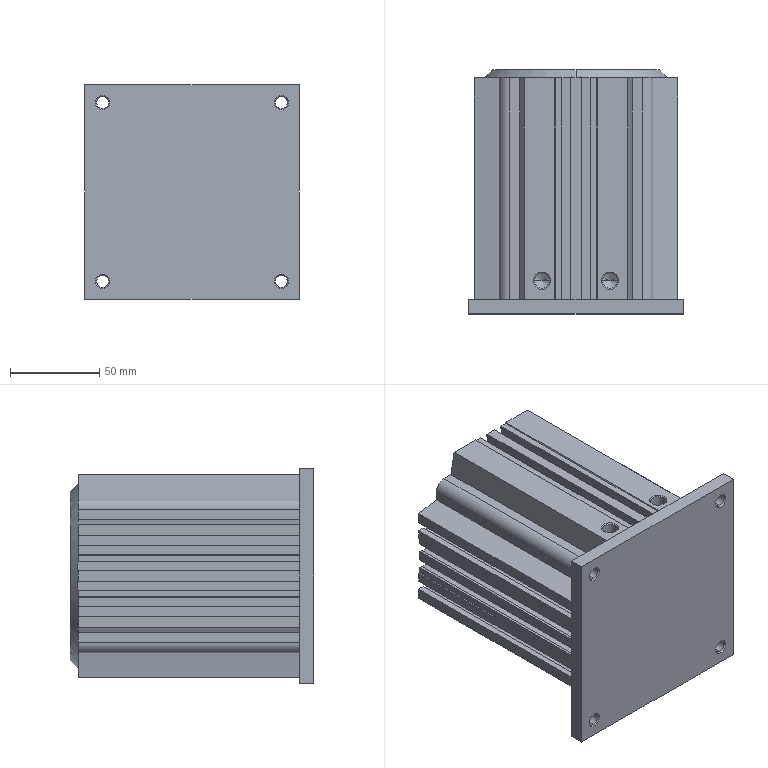Part | SolidWorks | features BaseBody 1 | 1 solid | 262 faces | box 120 x 136.5 x 120 mm | volume 637407 mm3 | plane 214 | cone 26 | cylinder 22 | commonest cylinder face diameters 6.647 x8 8.566 x4 12 x4 20 x2 40 x2 90 x2